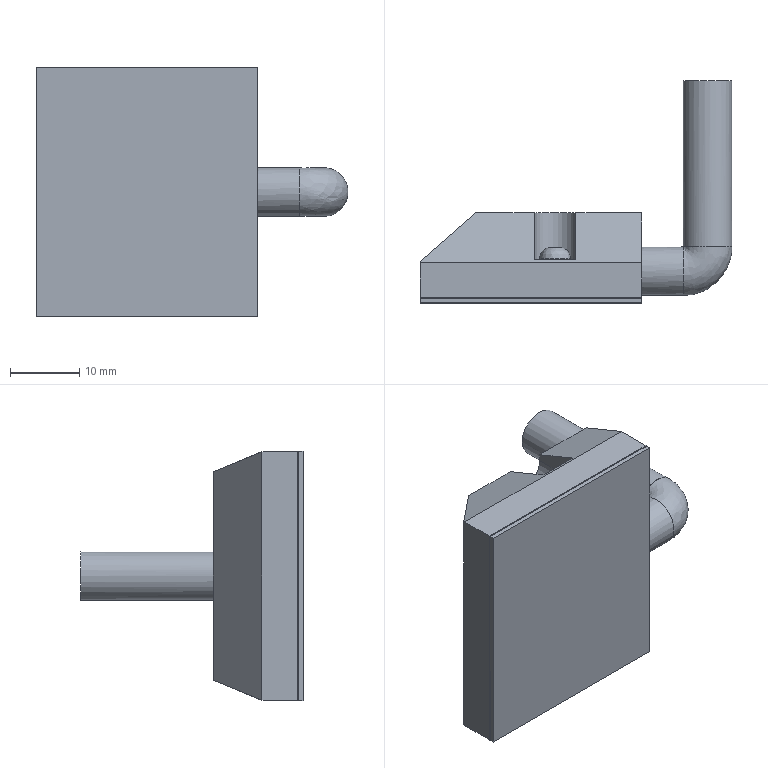Part | NX | 1 solid | 43 faces | box 45.035 x 32.1 x 36 mm | volume 14420 mm3 | plane 33 | cylinder 7 | spline 3 | commonest cylinder face diameters 4.5 x2 6 x2 7 x2 7.2 x1
STEP:
#1=CARTESIAN_POINT('',(-61.5,30.,-18.));
#2=VERTEX_POINT('',#1);
#3=CARTESIAN_POINT('',(-61.5,30.,18.));
#4=VERTEX_POINT('',#3);
#5=CARTESIAN_POINT('',(-61.5,30.,18.));
#6=DIRECTION('',(0.,0.,-1.));
#7=VECTOR('',#6,1000.);
#8=LINE('',#5,#7);
#9=EDGE_CURVE('',#2,#4,#8,.F.);
#10=ORIENTED_EDGE('',*,*,#9,.T.);
#11=CARTESIAN_POINT('',(-93.5,30.,18.));
#12=VERTEX_POINT('',#11);
#13=CARTESIAN_POINT('',(-61.5,30.,18.));
#14=DIRECTION('',(1.,0.,0.));
#15=VECTOR('',#14,1000.);
#16=LINE('',#13,#15);
#17=EDGE_CURVE('',#4,#12,#16,.F.);
#18=ORIENTED_EDGE('',*,*,#17,.T.);
#19=CARTESIAN_POINT('',(-93.5,30.,-18.));
#20=VERTEX_POINT('',#19);
#21=CARTESIAN_POINT('',(-93.5,30.,18.));
#22=DIRECTION('',(0.,0.,-1.));
#23=VECTOR('',#22,1000.);
#24=LINE('',#21,#23);
#25=EDGE_CURVE('',#12,#20,#24,.T.);
#26=ORIENTED_EDGE('',*,*,#25,.T.);
#27=CARTESIAN_POINT('',(-61.5,30.,-18.));
#28=DIRECTION('',(1.,0.,0.));
#29=VECTOR('',#28,1000.);
#30=LINE('',#27,#29);
#31=EDGE_CURVE('',#20,#2,#30,.T.);
#32=ORIENTED_EDGE('',*,*,#31,.T.);
#33=EDGE_LOOP('',(#10,#18,#26,#32));
#34=FACE_BOUND('',#33,.T.);
#35=CARTESIAN_POINT('',(-61.5,30.,18.));
#36=DIRECTION('',(0.,-1.,0.));
#37=DIRECTION('',(0.,0.,-1.));
#38=AXIS2_PLACEMENT_3D('',#35,#36,#37);
#39=PLANE('',#38);
#40=ADVANCED_FACE('',(#34),#39,.T.);
#41=CARTESIAN_POINT('',(-61.5,30.7,18.));
#42=VERTEX_POINT('',#41);
#43=CARTESIAN_POINT('',(-61.5,30.7,18.));
#44=DIRECTION('',(0.,1.,0.));
#45=VECTOR('',#44,1000.);
#46=LINE('',#43,#45);
#47=EDGE_CURVE('',#4,#42,#46,.T.);
#48=ORIENTED_EDGE('',*,*,#47,.T.);
#49=CARTESIAN_POINT('',(-93.5,30.7,18.));
#50=VERTEX_POINT('',#49);
#51=CARTESIAN_POINT('',(-61.5,30.7,18.));
#52=DIRECTION('',(1.,0.,0.));
#53=VECTOR('',#52,1000.);
#54=LINE('',#51,#53);
#55=EDGE_CURVE('',#42,#50,#54,.F.);
#56=ORIENTED_EDGE('',*,*,#55,.T.);
#57=CARTESIAN_POINT('',(-93.5,30.7,18.));
#58=DIRECTION('',(0.,1.,0.));
#59=VECTOR('',#58,1000.);
#60=LINE('',#57,#59);
#61=EDGE_CURVE('',#50,#12,#60,.F.);
#62=ORIENTED_EDGE('',*,*,#61,.T.);
#63=ORIENTED_EDGE('',*,*,#17,.F.);
#64=EDGE_LOOP('',(#48,#56,#62,#63));
#65=FACE_BOUND('',#64,.T.);
#66=CARTESIAN_POINT('',(-61.5,30.7,18.));
#67=DIRECTION('',(0.,0.,1.));
#68=DIRECTION('',(1.,0.,0.));
#69=AXIS2_PLACEMENT_3D('',#66,#67,#68);
#70=PLANE('',#69);
#71=ADVANCED_FACE('',(#65),#70,.T.);
#72=ORIENTED_EDGE('',*,*,#47,.F.);
#73=ORIENTED_EDGE('',*,*,#9,.F.);
#74=CARTESIAN_POINT('',(-61.5,30.7,-18.));
#75=VERTEX_POINT('',#74);
#76=CARTESIAN_POINT('',(-61.5,30.,-18.));
#77=DIRECTION('',(0.,1.,0.));
#78=VECTOR('',#77,1000.);
#79=LINE('',#76,#78);
#80=EDGE_CURVE('',#75,#2,#79,.F.);
#81=ORIENTED_EDGE('',*,*,#80,.F.);
#82=CARTESIAN_POINT('',(-61.5,30.7,0.));
#83=DIRECTION('',(0.,0.,1.));
#84=VECTOR('',#83,1000.);
#85=LINE('',#82,#84);
#86=EDGE_CURVE('',#42,#75,#85,.F.);
#87=ORIENTED_EDGE('',*,*,#86,.F.);
#88=EDGE_LOOP('',(#72,#73,#81,#87));
#89=FACE_BOUND('',#88,.T.);
#90=CARTESIAN_POINT('',(-61.5,30.,0.));
#91=DIRECTION('',(-1.,0.,0.));
#92=DIRECTION('',(0.,0.,1.));
#93=AXIS2_PLACEMENT_3D('',#90,#91,#92);
#94=PLANE('',#93);
#95=ADVANCED_FACE('',(#89),#94,.F.);
#96=ORIENTED_EDGE('',*,*,#80,.T.);
#97=ORIENTED_EDGE('',*,*,#31,.F.);
#98=CARTESIAN_POINT('',(-93.5,30.7,-18.));
#99=VERTEX_POINT('',#98);
#100=CARTESIAN_POINT('',(-93.5,30.,-18.));
#101=DIRECTION('',(0.,1.,0.));
#102=VECTOR('',#101,1000.);
#103=LINE('',#100,#102);
#104=EDGE_CURVE('',#20,#99,#103,.T.);
#105=ORIENTED_EDGE('',*,*,#104,.T.);
#106=CARTESIAN_POINT('',(-61.5,30.7,-18.));
#107=DIRECTION('',(-1.,0.,0.));
#108=VECTOR('',#107,1000.);
#109=LINE('',#106,#108);
#110=EDGE_CURVE('',#99,#75,#109,.F.);
#111=ORIENTED_EDGE('',*,*,#110,.T.);
#112=EDGE_LOOP('',(#96,#97,#105,#111));
#113=FACE_BOUND('',#112,.T.);
#114=CARTESIAN_POINT('',(-61.5,30.,-18.));
#115=DIRECTION('',(0.,0.,-1.));
#116=DIRECTION('',(-1.,0.,0.));
#117=AXIS2_PLACEMENT_3D('',#114,#115,#116);
#118=PLANE('',#117);
#119=ADVANCED_FACE('',(#113),#118,.T.);
#120=ORIENTED_EDGE('',*,*,#25,.F.);
#121=ORIENTED_EDGE('',*,*,#61,.F.);
#122=CARTESIAN_POINT('',(-93.5,30.7,0.));
#123=DIRECTION('',(0.,0.,1.));
#124=VECTOR('',#123,1000.);
#125=LINE('',#122,#124);
#126=EDGE_CURVE('',#50,#99,#125,.F.);
#127=ORIENTED_EDGE('',*,*,#126,.T.);
#128=ORIENTED_EDGE('',*,*,#104,.F.);
#129=EDGE_LOOP('',(#120,#121,#127,#128));
#130=FACE_BOUND('',#129,.T.);
#131=CARTESIAN_POINT('',(-93.5,30.,0.));
#132=DIRECTION('',(-1.,0.,0.));
#133=DIRECTION('',(0.,0.,1.));
#134=AXIS2_PLACEMENT_3D('',#131,#132,#133);
#135=PLANE('',#134);
#136=ADVANCED_FACE('',(#130),#135,.T.);
#137=ORIENTED_EDGE('',*,*,#86,.T.);
#138=ORIENTED_EDGE('',*,*,#110,.F.);
#139=ORIENTED_EDGE('',*,*,#126,.F.);
#140=ORIENTED_EDGE('',*,*,#55,.F.);
#141=EDGE_LOOP('',(#137,#138,#139,#140));
#142=FACE_BOUND('',#141,.T.);
#143=CARTESIAN_POINT('',(-61.6,30.7,17.9));
#144=VERTEX_POINT('',#143);
#145=CARTESIAN_POINT('',(-93.4,30.7,17.9));
#146=VERTEX_POINT('',#145);
#147=CARTESIAN_POINT('',(-61.5,30.7,17.9));
#148=DIRECTION('',(1.,0.,0.));
#149=VECTOR('',#148,1000.);
#150=LINE('',#147,#149);
#151=EDGE_CURVE('',#144,#146,#150,.F.);
#152=ORIENTED_EDGE('',*,*,#151,.T.);
#153=CARTESIAN_POINT('',(-93.4,30.7,-17.9));
#154=VERTEX_POINT('',#153);
#155=CARTESIAN_POINT('',(-93.4,30.7,-18.));
#156=DIRECTION('',(0.,0.,1.));
#157=VECTOR('',#156,1000.);
#158=LINE('',#155,#157);
#159=EDGE_CURVE('',#146,#154,#158,.F.);
#160=ORIENTED_EDGE('',*,*,#159,.T.);
#161=CARTESIAN_POINT('',(-61.6,30.7,-17.9));
#162=VERTEX_POINT('',#161);
#163=CARTESIAN_POINT('',(-61.5,30.7,-17.9));
#164=DIRECTION('',(1.,0.,0.));
#165=VECTOR('',#164,1000.);
#166=LINE('',#163,#165);
#167=EDGE_CURVE('',#154,#162,#166,.T.);
#168=ORIENTED_EDGE('',*,*,#167,.T.);
#169=CARTESIAN_POINT('',(-61.6,30.7,-18.));
#170=DIRECTION('',(0.,0.,1.));
#171=VECTOR('',#170,1000.);
#172=LINE('',#169,#171);
#173=EDGE_CURVE('',#162,#144,#172,.T.);
#174=ORIENTED_EDGE('',*,*,#173,.T.);
#175=EDGE_LOOP('',(#152,#160,#168,#174));
#176=FACE_BOUND('',#175,.T.);
#177=CARTESIAN_POINT('',(-61.5,30.7,-18.));
#178=DIRECTION('',(0.,1.,0.));
#179=DIRECTION('',(0.,0.,1.));
#180=AXIS2_PLACEMENT_3D('',#177,#178,#179);
#181=PLANE('',#180);
#182=ADVANCED_FACE('',(#142,#176),#181,.T.);
#183=CARTESIAN_POINT('',(-93.4,30.8,17.9));
#184=VERTEX_POINT('',#183);
#185=CARTESIAN_POINT('',(-93.4,30.,17.9));
#186=DIRECTION('',(0.,1.,0.));
#187=VECTOR('',#186,1000.);
#188=LINE('',#185,#187);
#189=EDGE_CURVE('',#146,#184,#188,.T.);
#190=ORIENTED_EDGE('',*,*,#189,.T.);
#191=CARTESIAN_POINT('',(-93.4,30.8,-17.9));
#192=VERTEX_POINT('',#191);
#193=CARTESIAN_POINT('',(-93.4,30.8,0.));
#194=DIRECTION('',(0.,0.,1.));
#195=VECTOR('',#194,1000.);
#196=LINE('',#193,#195);
#197=EDGE_CURVE('',#184,#192,#196,.F.);
#198=ORIENTED_EDGE('',*,*,#197,.T.);
#199=CARTESIAN_POINT('',(-93.4,30.,-17.9));
#200=DIRECTION('',(0.,1.,0.));
#201=VECTOR('',#200,1000.);
#202=LINE('',#199,#201);
#203=EDGE_CURVE('',#192,#154,#202,.F.);
#204=ORIENTED_EDGE('',*,*,#203,.T.);
#205=ORIENTED_EDGE('',*,*,#159,.F.);
#206=EDGE_LOOP('',(#190,#198,#204,#205));
#207=FACE_BOUND('',#206,.T.);
#208=CARTESIAN_POINT('',(-93.4,30.,0.));
#209=DIRECTION('',(-1.,0.,0.));
#210=DIRECTION('',(0.,0.,1.));
#211=AXIS2_PLACEMENT_3D('',#208,#209,#210);
#212=PLANE('',#211);
#213=ADVANCED_FACE('',(#207),#212,.T.);
#214=CARTESIAN_POINT('',(-61.6,30.8,17.9));
#215=VERTEX_POINT('',#214);
#216=CARTESIAN_POINT('',(-61.6,30.8,17.9));
#217=DIRECTION('',(0.,1.,0.));
#218=VECTOR('',#217,1000.);
#219=LINE('',#216,#218);
#220=EDGE_CURVE('',#144,#215,#219,.T.);
#221=ORIENTED_EDGE('',*,*,#220,.T.);
#222=CARTESIAN_POINT('',(-61.5,30.8,17.9));
#223=DIRECTION('',(1.,0.,0.));
#224=VECTOR('',#223,1000.);
#225=LINE('',#222,#224);
#226=EDGE_CURVE('',#215,#184,#225,.F.);
#227=ORIENTED_EDGE('',*,*,#226,.T.);
#228=ORIENTED_EDGE('',*,*,#189,.F.);
#229=ORIENTED_EDGE('',*,*,#151,.F.);
#230=EDGE_LOOP('',(#221,#227,#228,#229));
#231=FACE_BOUND('',#230,.T.);
#232=CARTESIAN_POINT('',(-61.5,30.8,17.9));
#233=DIRECTION('',(0.,0.,1.));
#234=DIRECTION('',(1.,0.,0.));
#235=AXIS2_PLACEMENT_3D('',#232,#233,#234);
#236=PLANE('',#235);
#237=ADVANCED_FACE('',(#231),#236,.T.);
#238=CARTESIAN_POINT('',(-61.6,30.8,-3.6));
#239=VERTEX_POINT('',#238);
#240=CARTESIAN_POINT('',(-61.6,30.8,-17.9));
#241=VERTEX_POINT('',#240);
#242=CARTESIAN_POINT('',(-61.6,30.8,0.));
#243=DIRECTION('',(0.,0.,1.));
#244=VECTOR('',#243,1000.);
#245=LINE('',#242,#244);
#246=EDGE_CURVE('',#239,#241,#245,.F.);
#247=ORIENTED_EDGE('',*,*,#246,.F.);
#248=CARTESIAN_POINT('',(-61.6,34.6,-3.6));
#249=VERTEX_POINT('',#248);
#250=CARTESIAN_POINT('',(-61.6,30.,-3.6));
#251=DIRECTION('',(0.,1.,0.));
#252=VECTOR('',#251,1000.);
#253=LINE('',#250,#252);
#254=EDGE_CURVE('',#249,#239,#253,.F.);
#255=ORIENTED_EDGE('',*,*,#254,.F.);
#256=CARTESIAN_POINT('',(-61.6,34.6,3.6));
#257=VERTEX_POINT('',#256);
#258=CARTESIAN_POINT('',(-61.6,34.6,0.));
#259=DIRECTION('',(1.,0.,0.));
#260=DIRECTION('',(0.,0.,-1.));
#261=AXIS2_PLACEMENT_3D('',#258,#259,#260);
#262=CIRCLE('',#261,3.6);
#263=EDGE_CURVE('',#257,#249,#262,.F.);
#264=ORIENTED_EDGE('',*,*,#263,.F.);
#265=CARTESIAN_POINT('',(-61.6,30.8,3.6));
#266=VERTEX_POINT('',#265);
#267=CARTESIAN_POINT('',(-61.6,30.,3.6));
#268=DIRECTION('',(0.,1.,0.));
#269=VECTOR('',#268,1000.);
#270=LINE('',#267,#269);
#271=EDGE_CURVE('',#266,#257,#270,.T.);
#272=ORIENTED_EDGE('',*,*,#271,.F.);
#273=CARTESIAN_POINT('',(-61.6,30.8,0.));
#274=DIRECTION('',(0.,0.,1.));
#275=VECTOR('',#274,1000.);
#276=LINE('',#273,#275);
#277=EDGE_CURVE('',#215,#266,#276,.F.);
#278=ORIENTED_EDGE('',*,*,#277,.F.);
#279=ORIENTED_EDGE('',*,*,#220,.F.);
#280=ORIENTED_EDGE('',*,*,#173,.F.);
#281=CARTESIAN_POINT('',(-61.6,30.,-17.9));
#282=DIRECTION('',(0.,1.,0.));
#283=VECTOR('',#282,1000.);
#284=LINE('',#281,#283);
#285=EDGE_CURVE('',#241,#162,#284,.F.);
#286=ORIENTED_EDGE('',*,*,#285,.F.);
#287=EDGE_LOOP('',(#247,#255,#264,#272,#278,#279,#280,#286));
#288=FACE_BOUND('',#287,.T.);
#289=CARTESIAN_POINT('',(-61.6,34.6,-3.5));
#290=VERTEX_POINT('',#289);
#291=CARTESIAN_POINT('',(-61.6,34.6,0.));
#292=DIRECTION('',(1.,0.,0.));
#293=DIRECTION('',(0.,0.,-1.));
#294=AXIS2_PLACEMENT_3D('',#291,#292,#293);
#295=CIRCLE('',#294,3.5);
#296=EDGE_CURVE('',#290,#290,#295,.T.);
#297=ORIENTED_EDGE('',*,*,#296,.F.);
#298=EDGE_LOOP('',(#297));
#299=FACE_BOUND('',#298,.T.);
#300=CARTESIAN_POINT('',(-61.6,30.,0.));
#301=DIRECTION('',(-1.,0.,0.));
#302=DIRECTION('',(0.,0.,1.));
#303=AXIS2_PLACEMENT_3D('',#300,#301,#302);
#304=PLANE('',#303);
#305=ADVANCED_FACE('',(#288,#299),#304,.F.);
#306=ORIENTED_EDGE('',*,*,#285,.T.);
#307=ORIENTED_EDGE('',*,*,#167,.F.);
#308=ORIENTED_EDGE('',*,*,#203,.F.);
#309=CARTESIAN_POINT('',(-61.5,30.8,-17.9));
#310=DIRECTION('',(1.,0.,0.));
#311=VECTOR('',#310,1000.);
#312=LINE('',#309,#311);
#313=EDGE_CURVE('',#192,#241,#312,.T.);
#314=ORIENTED_EDGE('',*,*,#313,.T.);
#315=EDGE_LOOP('',(#306,#307,#308,#314));
#316=FACE_BOUND('',#315,.T.);
#317=CARTESIAN_POINT('',(-61.5,30.7,-17.9));
#318=DIRECTION('',(0.,0.,-1.));
#319=DIRECTION('',(0.,1.,0.));
#320=AXIS2_PLACEMENT_3D('',#317,#318,#319);
#321=PLANE('',#320);
#322=ADVANCED_FACE('',(#316),#321,.T.);
#323=CARTESIAN_POINT('',(-93.5,30.8,-18.));
#324=VERTEX_POINT('',#323);
#325=CARTESIAN_POINT('',(-61.5,30.8,-18.));
#326=VERTEX_POINT('',#325);
#327=CARTESIAN_POINT('',(-61.5,30.8,-18.));
#328=DIRECTION('',(1.,0.,0.));
#329=VECTOR('',#328,1000.);
#330=LINE('',#327,#329);
#331=EDGE_CURVE('',#324,#326,#330,.T.);
#332=ORIENTED_EDGE('',*,*,#331,.T.);
#333=CARTESIAN_POINT('',(-61.5,30.8,-3.6));
#334=VERTEX_POINT('',#333);
#335=CARTESIAN_POINT('',(-61.5,30.8,-17.9));
#336=DIRECTION('',(0.,0.,-1.));
#337=VECTOR('',#336,1000.);
#338=LINE('',#335,#337);
#339=EDGE_CURVE('',#326,#334,#338,.F.);
#340=ORIENTED_EDGE('',*,*,#339,.T.);
#341=CARTESIAN_POINT('',(-61.5,30.8,-3.6));
#342=DIRECTION('',(1.,0.,0.));
#343=VECTOR('',#342,1000.);
#344=LINE('',#341,#343);
#345=EDGE_CURVE('',#334,#239,#344,.F.);
#346=ORIENTED_EDGE('',*,*,#345,.T.);
#347=ORIENTED_EDGE('',*,*,#246,.T.);
#348=ORIENTED_EDGE('',*,*,#313,.F.);
#349=ORIENTED_EDGE('',*,*,#197,.F.);
#350=ORIENTED_EDGE('',*,*,#226,.F.);
#351=ORIENTED_EDGE('',*,*,#277,.T.);
#352=CARTESIAN_POINT('',(-61.5,30.8,3.6));
#353=VERTEX_POINT('',#352);
#354=CARTESIAN_POINT('',(-61.5,30.8,3.6));
#355=DIRECTION('',(1.,0.,0.));
#356=VECTOR('',#355,1000.);
#357=LINE('',#354,#356);
#358=EDGE_CURVE('',#266,#353,#357,.T.);
#359=ORIENTED_EDGE('',*,*,#358,.T.);
#360=CARTESIAN_POINT('',(-61.5,30.8,18.));
#361=VERTEX_POINT('',#360);
#362=CARTESIAN_POINT('',(-61.5,30.8,-17.9));
#363=DIRECTION('',(0.,0.,-1.));
#364=VECTOR('',#363,1000.);
#365=LINE('',#362,#364);
#366=EDGE_CURVE('',#353,#361,#365,.F.);
#367=ORIENTED_EDGE('',*,*,#366,.T.);
#368=CARTESIAN_POINT('',(-93.5,30.8,18.));
#369=VERTEX_POINT('',#368);
#370=CARTESIAN_POINT('',(-61.5,30.8,18.));
#371=DIRECTION('',(1.,0.,0.));
#372=VECTOR('',#371,1000.);
#373=LINE('',#370,#372);
#374=EDGE_CURVE('',#361,#369,#373,.F.);
#375=ORIENTED_EDGE('',*,*,#374,.T.);
#376=CARTESIAN_POINT('',(-93.5,30.8,-17.9));
#377=DIRECTION('',(0.,0.,-1.));
#378=VECTOR('',#377,1000.);
#379=LINE('',#376,#378);
#380=EDGE_CURVE('',#369,#324,#379,.T.);
#381=ORIENTED_EDGE('',*,*,#380,.T.);
#382=EDGE_LOOP('',(#332,#340,#346,#347,#348,#349,#350,#351,#359,#367,#375,#381));
#383=FACE_BOUND('',#382,.T.);
#384=CARTESIAN_POINT('',(-61.5,30.8,-17.9));
#385=DIRECTION('',(0.,-1.,0.));
#386=DIRECTION('',(0.,0.,-1.));
#387=AXIS2_PLACEMENT_3D('',#384,#385,#386);
#388=PLANE('',#387);
#389=ADVANCED_FACE('',(#383),#388,.T.);
#390=ORIENTED_EDGE('',*,*,#345,.F.);
#391=CARTESIAN_POINT('',(-61.5,34.6,-3.6));
#392=VERTEX_POINT('',#391);
#393=CARTESIAN_POINT('',(-61.5,30.8,-3.6));
#394=DIRECTION('',(0.,1.,0.));
#395=VECTOR('',#394,1000.);
#396=LINE('',#393,#395);
#397=EDGE_CURVE('',#392,#334,#396,.F.);
#398=ORIENTED_EDGE('',*,*,#397,.F.);
#399=CARTESIAN_POINT('',(-61.5,34.6,-3.6));
#400=DIRECTION('',(-1.,0.,0.));
#401=VECTOR('',#400,1000.);
#402=LINE('',#399,#401);
#403=EDGE_CURVE('',#249,#392,#402,.F.);
#404=ORIENTED_EDGE('',*,*,#403,.F.);
#405=ORIENTED_EDGE('',*,*,#254,.T.);
#406=EDGE_LOOP('',(#390,#398,#404,#405));
#407=FACE_BOUND('',#406,.T.);
#408=CARTESIAN_POINT('',(-61.5,30.8,-3.6));
#409=DIRECTION('',(0.,0.,-1.));
#410=DIRECTION('',(-1.,0.,0.));
#411=AXIS2_PLACEMENT_3D('',#408,#409,#410);
#412=PLANE('',#411);
#413=ADVANCED_FACE('',(#407),#412,.F.);
#414=ORIENTED_EDGE('',*,*,#403,.T.);
#415=CARTESIAN_POINT('',(-61.5,34.6,3.6));
#416=VERTEX_POINT('',#415);
#417=CARTESIAN_POINT('',(-61.5,34.6,0.));
#418=DIRECTION('',(1.,0.,0.));
#419=DIRECTION('',(0.,0.,-1.));
#420=AXIS2_PLACEMENT_3D('',#417,#418,#419);
#421=CIRCLE('',#420,3.6);
#422=EDGE_CURVE('',#416,#392,#421,.F.);
#423=ORIENTED_EDGE('',*,*,#422,.F.);
#424=CARTESIAN_POINT('',(-61.5,34.6,3.6));
#425=DIRECTION('',(1.,0.,0.));
#426=VECTOR('',#425,1000.);
#427=LINE('',#424,#426);
#428=EDGE_CURVE('',#257,#416,#427,.T.);
#429=ORIENTED_EDGE('',*,*,#428,.F.);
#430=ORIENTED_EDGE('',*,*,#263,.T.);
#431=EDGE_LOOP('',(#414,#423,#429,#430));
#432=FACE_BOUND('',#431,.T.);
#433=CARTESIAN_POINT('',(-61.5,34.6,0.));
#434=DIRECTION('',(1.,0.,0.));
#435=DIRECTION('',(0.,0.,-1.));
#436=AXIS2_PLACEMENT_3D('',#433,#434,#435);
#437=CYLINDRICAL_SURFACE('',#436,3.6);
#438=ADVANCED_FACE('',(#432),#437,.F.);
#439=ORIENTED_EDGE('',*,*,#428,.T.);
#440=CARTESIAN_POINT('',(-61.5,34.6,3.6));
#441=DIRECTION('',(0.,1.,0.));
#442=VECTOR('',#441,1000.);
#443=LINE('',#440,#442);
#444=EDGE_CURVE('',#353,#416,#443,.T.);
#445=ORIENTED_EDGE('',*,*,#444,.F.);
#446=ORIENTED_EDGE('',*,*,#358,.F.);
#447=ORIENTED_EDGE('',*,*,#271,.T.);
#448=EDGE_LOOP('',(#439,#445,#446,#447));
#449=FACE_BOUND('',#448,.T.);
#450=CARTESIAN_POINT('',(-61.5,34.6,3.6));
#451=DIRECTION('',(0.,0.,1.));
#452=DIRECTION('',(1.,0.,0.));
#453=AXIS2_PLACEMENT_3D('',#450,#451,#452);
#454=PLANE('',#453);
#455=ADVANCED_FACE('',(#449),#454,.F.);
#456=CARTESIAN_POINT('',(-55.5,38.1,0.));
#457=VERTEX_POINT('',#456);
#458=CARTESIAN_POINT('',(-55.5,34.6,0.));
#459=DIRECTION('',(1.,0.,0.));
#460=DIRECTION('',(0.,0.,-1.));
#461=AXIS2_PLACEMENT_3D('',#458,#459,#460);
#462=CIRCLE('',#461,3.5);
#463=EDGE_CURVE('',#457,#457,#462,.F.);
#464=ORIENTED_EDGE('',*,*,#463,.T.);
#465=EDGE_LOOP('',(#464));
#466=FACE_BOUND('',#465,.T.);
#467=ORIENTED_EDGE('',*,*,#296,.T.);
#468=EDGE_LOOP('',(#467));
#469=FACE_BOUND('',#468,.T.);
#470=CARTESIAN_POINT('',(-55.5,34.6,0.));
#471=DIRECTION('',(1.,0.,0.));
#472=DIRECTION('',(0.,0.,-1.));
#473=AXIS2_PLACEMENT_3D('',#470,#471,#472);
#474=CYLINDRICAL_SURFACE('',#473,3.5);
#475=ADVANCED_FACE('',(#466,#469),#474,.T.);
#476=ORIENTED_EDGE('',*,*,#339,.F.);
#477=CARTESIAN_POINT('',(-61.5,35.8,-18.));
#478=VERTEX_POINT('',#477);
#479=CARTESIAN_POINT('',(-61.5,30.,-18.));
#480=DIRECTION('',(0.,1.,0.));
#481=VECTOR('',#480,1000.);
#482=LINE('',#479,#481);
#483=EDGE_CURVE('',#478,#326,#482,.F.);
#484=ORIENTED_EDGE('',*,*,#483,.F.);
#485=CARTESIAN_POINT('',(-61.5,43.,-15.041));
#486=VERTEX_POINT('',#485);
#487=CARTESIAN_POINT('',(-61.5,43.,-15.041));
#488=DIRECTION('',(0.,-0.9249,-0.3801));
#489=VECTOR('',#488,1000.);
#490=LINE('',#487,#489);
#491=EDGE_CURVE('',#486,#478,#490,.T.);
#492=ORIENTED_EDGE('',*,*,#491,.F.);
#493=CARTESIAN_POINT('',(-61.5,43.,15.041));
#494=VERTEX_POINT('',#493);
#495=CARTESIAN_POINT('',(-61.5,43.,0.));
#496=DIRECTION('',(0.,0.,1.));
#497=VECTOR('',#496,1000.);
#498=LINE('',#495,#497);
#499=EDGE_CURVE('',#494,#486,#498,.F.);
#500=ORIENTED_EDGE('',*,*,#499,.F.);
#501=CARTESIAN_POINT('',(-61.5,35.8,18.));
#502=VERTEX_POINT('',#501);
#503=CARTESIAN_POINT('',(-61.5,35.8,18.));
#504=DIRECTION('',(0.,0.9249,-0.3801));
#505=VECTOR('',#504,1000.);
#506=LINE('',#503,#505);
#507=EDGE_CURVE('',#502,#494,#506,.T.);
#508=ORIENTED_EDGE('',*,*,#507,.F.);
#509=CARTESIAN_POINT('',(-61.5,30.,18.));
#510=DIRECTION('',(0.,1.,0.));
#511=VECTOR('',#510,1000.);
#512=LINE('',#509,#511);
#513=EDGE_CURVE('',#361,#502,#512,.T.);
#514=ORIENTED_EDGE('',*,*,#513,.F.);
#515=ORIENTED_EDGE('',*,*,#366,.F.);
#516=ORIENTED_EDGE('',*,*,#444,.T.);
#517=ORIENTED_EDGE('',*,*,#422,.T.);
#518=ORIENTED_EDGE('',*,*,#397,.T.);
#519=EDGE_LOOP('',(#476,#484,#492,#500,#508,#514,#515,#516,#517,#518));
#520=FACE_BOUND('',#519,.T.);
#521=CARTESIAN_POINT('',(-61.5,30.,0.));
#522=DIRECTION('',(-1.,0.,0.));
#523=DIRECTION('',(0.,0.,1.));
#524=AXIS2_PLACEMENT_3D('',#521,#522,#523);
#525=PLANE('',#524);
#526=ADVANCED_FACE('',(#520),#525,.F.);
#527=ORIENTED_EDGE('',*,*,#483,.T.);
#528=ORIENTED_EDGE('',*,*,#331,.F.);
#529=CARTESIAN_POINT('',(-93.5,35.8,-18.));
#530=VERTEX_POINT('',#529);
#531=CARTESIAN_POINT('',(-93.5,30.8,-18.));
#532=DIRECTION('',(0.,1.,0.));
#533=VECTOR('',#532,1000.);
#534=LINE('',#531,#533);
#535=EDGE_CURVE('',#324,#530,#534,.T.);
#536=ORIENTED_EDGE('',*,*,#535,.T.);
#537=CARTESIAN_POINT('',(-61.5,35.8,-18.));
#538=DIRECTION('',(-1.,0.,0.));
#539=VECTOR('',#538,1000.);
#540=LINE('',#537,#539);
#541=EDGE_CURVE('',#530,#478,#540,.F.);
#542=ORIENTED_EDGE('',*,*,#541,.T.);
#543=EDGE_LOOP('',(#527,#528,#536,#542));
#544=FACE_BOUND('',#543,.T.);
#545=CARTESIAN_POINT('',(-61.5,30.8,-18.));
#546=DIRECTION('',(0.,0.,-1.));
#547=DIRECTION('',(-1.,0.,0.));
#548=AXIS2_PLACEMENT_3D('',#545,#546,#547);
#549=PLANE('',#548);
#550=ADVANCED_FACE('',(#544),#549,.T.);
#551=CARTESIAN_POINT('',(-93.5,35.8,18.));
#552=VERTEX_POINT('',#551);
#553=CARTESIAN_POINT('',(-93.5,30.,18.));
#554=DIRECTION('',(0.,1.,0.));
#555=VECTOR('',#554,1000.);
#556=LINE('',#553,#555);
#557=EDGE_CURVE('',#369,#552,#556,.T.);
#558=ORIENTED_EDGE('',*,*,#557,.T.);
#559=CARTESIAN_POINT('',(-93.5,36.,17.918));
#560=VERTEX_POINT('',#559);
#561=CARTESIAN_POINT('',(-93.5,35.8,18.));
#562=DIRECTION('',(0.,0.9249,-0.3801));
#563=VECTOR('',#562,1000.);
#564=LINE('',#561,#563);
#565=EDGE_CURVE('',#552,#560,#564,.T.);
#566=ORIENTED_EDGE('',*,*,#565,.T.);
#567=CARTESIAN_POINT('',(-93.5,36.,-17.918));
#568=VERTEX_POINT('',#567);
#569=CARTESIAN_POINT('',(-93.5,36.,0.));
#570=DIRECTION('',(0.,0.,1.));
#571=VECTOR('',#570,1000.);
#572=LINE('',#569,#571);
#573=EDGE_CURVE('',#560,#568,#572,.F.);
#574=ORIENTED_EDGE('',*,*,#573,.T.);
#575=CARTESIAN_POINT('',(-93.5,36.,-17.918));
#576=DIRECTION('',(0.,-0.9249,-0.3801));
#577=VECTOR('',#576,1000.);
#578=LINE('',#575,#577);
#579=EDGE_CURVE('',#568,#530,#578,.T.);
#580=ORIENTED_EDGE('',*,*,#579,.T.);
#581=ORIENTED_EDGE('',*,*,#535,.F.);
#582=ORIENTED_EDGE('',*,*,#380,.F.);
#583=EDGE_LOOP('',(#558,#566,#574,#580,#581,#582));
#584=FACE_BOUND('',#583,.T.);
#585=CARTESIAN_POINT('',(-93.5,30.,0.));
#586=DIRECTION('',(-1.,0.,0.));
#587=DIRECTION('',(0.,0.,1.));
#588=AXIS2_PLACEMENT_3D('',#585,#586,#587);
#589=PLANE('',#588);
#590=ADVANCED_FACE('',(#584),#589,.T.);
#591=ORIENTED_EDGE('',*,*,#513,.T.);
#592=CARTESIAN_POINT('',(-61.5,35.8,18.));
#593=DIRECTION('',(1.,0.,0.));
#594=VECTOR('',#593,1000.);
#595=LINE('',#592,#594);
#596=EDGE_CURVE('',#502,#552,#595,.F.);
#597=ORIENTED_EDGE('',*,*,#596,.T.);
#598=ORIENTED_EDGE('',*,*,#557,.F.);
#599=ORIENTED_EDGE('',*,*,#374,.F.);
#600=EDGE_LOOP('',(#591,#597,#598,#599));
#601=FACE_BOUND('',#600,.T.);
#602=CARTESIAN_POINT('',(-61.5,35.8,18.));
#603=DIRECTION('',(0.,0.,1.));
#604=DIRECTION('',(1.,0.,0.));
#605=AXIS2_PLACEMENT_3D('',#602,#603,#604);
#606=PLANE('',#605);
#607=ADVANCED_FACE('',(#601),#606,.T.);
#608=CARTESIAN_POINT('',(-51.983,38.135,-3.5));
#609=VERTEX_POINT('',#608);
#610=CARTESIAN_POINT('',(-51.991,38.1,-3.5));
#611=VERTEX_POINT('',#610);
#612=CARTESIAN_POINT('',(-51.982,38.135,-3.5));
#613=CARTESIAN_POINT('',(-51.983,38.123,-3.5));
#614=CARTESIAN_POINT('',(-51.983,38.112,-3.5));
#615=CARTESIAN_POINT('',(-51.983,38.1,-3.5));
#616=B_SPLINE_CURVE_WITH_KNOTS('',3,(#612,#613,#614,#615),.UNSPECIFIED.,.F.,.F.,(4,4),(0.,1.),.UNSPECIFIED.);
#617=EDGE_CURVE('',#609,#611,#616,.T.);
#618=ORIENTED_EDGE('',*,*,#617,.F.);
#619=CARTESIAN_POINT('',(-51.983,38.135,3.5));
#620=VERTEX_POINT('',#619);
#621=CARTESIAN_POINT('',(-51.983,38.135,-3.5));
#622=CARTESIAN_POINT('',(-51.055,38.135,-3.505));
#623=CARTESIAN_POINT('',(-49.234,38.135,-2.753));
#624=CARTESIAN_POINT('',(-48.081,38.135,0.0008832));
#625=CARTESIAN_POINT('',(-49.231,38.135,2.749));
#626=CARTESIAN_POINT('',(-51.055,38.135,3.505));
#627=CARTESIAN_POINT('',(-51.983,38.135,3.5));
#628=B_SPLINE_CURVE_WITH_KNOTS('',3,(#621,#622,#623,#624,#625,#626,#627),.UNSPECIFIED.,.F.,.F.,(4,1,1,1,4),(0.,0.002743,0.005485,0.008228,0.01097),.UNSPECIFIED.);
#629=EDGE_CURVE('',#609,#620,#628,.T.);
#630=ORIENTED_EDGE('',*,*,#629,.T.);
#631=CARTESIAN_POINT('',(-51.991,38.1,3.5));
#632=VERTEX_POINT('',#631);
#633=CARTESIAN_POINT('',(-51.983,38.1,3.5));
#634=CARTESIAN_POINT('',(-51.983,38.112,3.5));
#635=CARTESIAN_POINT('',(-51.983,38.123,3.5));
#636=CARTESIAN_POINT('',(-51.983,38.135,3.5));
#637=B_SPLINE_CURVE_WITH_KNOTS('',3,(#633,#634,#635,#636),.UNSPECIFIED.,.F.,.F.,(4,4),(0.,1.),.UNSPECIFIED.);
#638=EDGE_CURVE('',#632,#620,#637,.T.);
#639=ORIENTED_EDGE('',*,*,#638,.F.);
#640=CARTESIAN_POINT('',(-51.991,38.1,3.5));
#641=CARTESIAN_POINT('',(-52.912,38.1,3.493));
#642=CARTESIAN_POINT('',(-54.252,38.1,2.916));
#643=CARTESIAN_POINT('',(-55.292,38.1,1.371));
#644=CARTESIAN_POINT('',(-55.455,38.1,0.4516));
#645=CARTESIAN_POINT('',(-55.5,38.1,0.));
#646=B_SPLINE_CURVE_WITH_KNOTS('',3,(#640,#641,#642,#643,#644,#645),.UNSPECIFIED.,.F.,.F.,(4,1,1,4),(0.,0.002723,0.004084,0.005446),.UNSPECIFIED.);
#647=EDGE_CURVE('',#632,#457,#646,.T.);
#648=ORIENTED_EDGE('',*,*,#647,.T.);
#649=ORIENTED_EDGE('',*,*,#463,.F.);
#650=CARTESIAN_POINT('',(-52.,38.1,-3.5));
#651=CARTESIAN_POINT('',(-52.461,38.1,-3.495));
#652=CARTESIAN_POINT('',(-53.359,38.1,-3.306));
#653=CARTESIAN_POINT('',(-54.516,38.1,-2.529));
#654=CARTESIAN_POINT('',(-55.155,38.1,-1.557));
#655=CARTESIAN_POINT('',(-55.39,38.1,-0.8039));
#656=CARTESIAN_POINT('',(-55.469,38.1,-0.3137));
#657=CARTESIAN_POINT('',(-55.485,38.1,-0.1451));
#658=CARTESIAN_POINT('',(-55.5,38.1,0.));
#659=B_SPLINE_CURVE_WITH_KNOTS('',3,(#650,#651,#652,#653,#654,#655,#656,#657,#658),.UNSPECIFIED.,.F.,.F.,(4,1,1,1,1,1,4),(0.003134,0.2524,0.5016,0.7508,0.8754,0.9377,1.),.UNSPECIFIED.);
#660=EDGE_CURVE('',#457,#611,#659,.F.);
#661=ORIENTED_EDGE('',*,*,#660,.T.);
#662=EDGE_LOOP('',(#618,#630,#639,#648,#649,#661));
#663=FACE_BOUND('',#662,.T.);
#664=CARTESIAN_POINT('',(-55.5,31.857,2.743));
#665=CARTESIAN_POINT('',(-51.795,31.857,2.743));
#666=CARTESIAN_POINT('',(-49.188,34.489,2.743));
#667=CARTESIAN_POINT('',(-49.223,38.194,2.743));
#668=CARTESIAN_POINT('',(-55.5,30.721,0.));
#669=CARTESIAN_POINT('',(-51.125,30.721,0.));
#670=CARTESIAN_POINT('',(-48.045,33.83,0.));
#671=CARTESIAN_POINT('',(-48.087,38.205,0.));
#672=CARTESIAN_POINT('',(-55.5,31.857,-2.743));
#673=CARTESIAN_POINT('',(-51.795,31.857,-2.743));
#674=CARTESIAN_POINT('',(-49.188,34.489,-2.743));
#675=CARTESIAN_POINT('',(-49.223,38.194,-2.743));
#676=CARTESIAN_POINT('',(-55.5,34.6,-3.879));
#677=CARTESIAN_POINT('',(-53.414,34.6,-3.879));
#678=CARTESIAN_POINT('',(-51.945,36.082,-3.879));
#679=CARTESIAN_POINT('',(-51.965,38.168,-3.879));
#680=CARTESIAN_POINT('',(-55.5,37.343,-2.743));
#681=CARTESIAN_POINT('',(-55.032,37.343,-2.743));
#682=CARTESIAN_POINT('',(-54.703,37.675,-2.743));
#683=CARTESIAN_POINT('',(-54.708,38.142,-2.743));
#684=CARTESIAN_POINT('',(-55.5,38.479,0.));
#685=CARTESIAN_POINT('',(-55.703,38.479,0.));
#686=CARTESIAN_POINT('',(-55.846,38.335,0.));
#687=CARTESIAN_POINT('',(-55.844,38.132,0.));
#688=CARTESIAN_POINT('',(-55.5,37.343,2.743));
#689=CARTESIAN_POINT('',(-55.032,37.343,2.743));
#690=CARTESIAN_POINT('',(-54.703,37.675,2.743));
#691=CARTESIAN_POINT('',(-54.708,38.142,2.743));
#692=CARTESIAN_POINT('',(-55.5,34.6,3.879));
#693=CARTESIAN_POINT('',(-53.414,34.6,3.879));
#694=CARTESIAN_POINT('',(-51.945,36.082,3.879));
#695=CARTESIAN_POINT('',(-51.965,38.168,3.879));
#696=CARTESIAN_POINT('',(-55.5,31.857,2.743));
#697=CARTESIAN_POINT('',(-51.795,31.857,2.743));
#698=CARTESIAN_POINT('',(-49.188,34.489,2.743));
#699=CARTESIAN_POINT('',(-49.223,38.194,2.743));
#700=CARTESIAN_POINT('',(-55.5,30.721,0.));
#701=CARTESIAN_POINT('',(-51.125,30.721,0.));
#702=CARTESIAN_POINT('',(-48.045,33.83,0.));
#703=CARTESIAN_POINT('',(-48.087,38.205,0.));
#704=CARTESIAN_POINT('',(-55.5,31.857,-2.743));
#705=CARTESIAN_POINT('',(-51.795,31.857,-2.743));
#706=CARTESIAN_POINT('',(-49.188,34.489,-2.743));
#707=CARTESIAN_POINT('',(-49.223,38.194,-2.743));
#708=(BOUNDED_SURFACE()B_SPLINE_SURFACE(3,3,((#664,#665,#666,#667),(#668,#669,#670,#671),(#672,#673,#674,#675),(#676,#677,#678,#679),(#680,#681,#682,#683),(#684,#685,#686,#687),(#688,#689,#690,#691),(#692,#693,#694,#695),(#696,#697,#698,#699),(#700,#701,#702,#703),(#704,#705,#706,#707)),.SURF_OF_REVOLUTION.,.T.,.F.,.F.)B_SPLINE_SURFACE_WITH_KNOTS((1,1,1,1,1,1,1,1,1,1,1,1,1,1,1),(4,4),(-2.356,-1.571,-0.7854,0.,0.7854,1.571,2.356,3.142,3.927,4.712,5.498,6.283,7.069,7.854,8.639),(0.,1.),.UNSPECIFIED.)GEOMETRIC_REPRESENTATION_ITEM()RATIONAL_B_SPLINE_SURFACE(((1.,0.8025,0.8025,1.),(1.,0.8025,0.8025,1.),(1.,0.8025,0.8025,1.),(1.,0.8025,0.8025,1.),(1.,0.8025,0.8025,1.),(1.,0.8025,0.8025,1.),(1.,0.8025,0.8025,1.),(1.,0.8025,0.8025,1.),(1.,0.8025,0.8025,1.),(1.,0.8025,0.8025,1.),(1.,0.8025,0.8025,1.)))REPRESENTATION_ITEM('')SURFACE());
#709=ADVANCED_FACE('',(#663),#708,.T.);
#710=CARTESIAN_POINT('',(-77.,43.,-15.041));
#711=VERTEX_POINT('',#710);
#712=CARTESIAN_POINT('',(-77.,36.3,-17.795));
#713=VERTEX_POINT('',#712);
#714=CARTESIAN_POINT('',(-77.,35.8,-18.));
#715=DIRECTION('',(0.,0.9249,0.3801));
#716=VECTOR('',#715,1000.);
#717=LINE('',#714,#716);
#718=EDGE_CURVE('',#711,#713,#717,.F.);
#719=ORIENTED_EDGE('',*,*,#718,.T.);
#720=CARTESIAN_POINT('',(-71.,36.3,-17.795));
#721=VERTEX_POINT('',#720);
#722=CARTESIAN_POINT('',(-61.5,36.3,-17.795));
#723=DIRECTION('',(1.,0.,0.));
#724=VECTOR('',#723,1000.);
#725=LINE('',#722,#724);
#726=EDGE_CURVE('',#713,#721,#725,.T.);
#727=ORIENTED_EDGE('',*,*,#726,.T.);
#728=CARTESIAN_POINT('',(-71.,43.,-15.041));
#729=VERTEX_POINT('',#728);
#730=CARTESIAN_POINT('',(-71.,35.8,-18.));
#731=DIRECTION('',(0.,0.9249,0.3801));
#732=VECTOR('',#731,1000.);
#733=LINE('',#730,#732);
#734=EDGE_CURVE('',#721,#729,#733,.T.);
#735=ORIENTED_EDGE('',*,*,#734,.T.);
#736=CARTESIAN_POINT('',(-61.5,43.,-15.041));
#737=DIRECTION('',(1.,0.,0.));
#738=VECTOR('',#737,1000.);
#739=LINE('',#736,#738);
#740=EDGE_CURVE('',#729,#486,#739,.T.);
#741=ORIENTED_EDGE('',*,*,#740,.T.);
#742=ORIENTED_EDGE('',*,*,#491,.T.);
#743=ORIENTED_EDGE('',*,*,#541,.F.);
#744=ORIENTED_EDGE('',*,*,#579,.F.);
#745=CARTESIAN_POINT('',(-85.5,43.,-15.041));
#746=VERTEX_POINT('',#745);
#747=CARTESIAN_POINT('',(-93.5,36.,-17.918));
#748=DIRECTION('',(0.7264,0.6356,0.2612));
#749=VECTOR('',#748,1000.);
#750=LINE('',#747,#749);
#751=EDGE_CURVE('',#568,#746,#750,.T.);
#752=ORIENTED_EDGE('',*,*,#751,.T.);
#753=CARTESIAN_POINT('',(-61.5,43.,-15.041));
#754=DIRECTION('',(1.,0.,0.));
#755=VECTOR('',#754,1000.);
#756=LINE('',#753,#755);
#757=EDGE_CURVE('',#746,#711,#756,.T.);
#758=ORIENTED_EDGE('',*,*,#757,.T.);
#759=EDGE_LOOP('',(#719,#727,#735,#741,#742,#743,#744,#752,#758));
#760=FACE_BOUND('',#759,.T.);
#761=CARTESIAN_POINT('',(-61.5,35.8,-18.));
#762=DIRECTION('',(0.,0.3801,-0.9249));
#763=DIRECTION('',(0.,0.9249,0.3801));
#764=AXIS2_PLACEMENT_3D('',#761,#762,#763);
#765=PLANE('',#764);
#766=ADVANCED_FACE('',(#760),#765,.T.);
#767=CARTESIAN_POINT('',(-85.5,43.,15.041));
#768=VERTEX_POINT('',#767);
#769=CARTESIAN_POINT('',(-85.5,43.,-15.041));
#770=DIRECTION('',(0.,0.,1.));
#771=VECTOR('',#770,1000.);
#772=LINE('',#769,#771);
#773=EDGE_CURVE('',#746,#768,#772,.T.);
#774=ORIENTED_EDGE('',*,*,#773,.T.);
#775=CARTESIAN_POINT('',(-77.,43.,15.041));
#776=VERTEX_POINT('',#775);
#777=CARTESIAN_POINT('',(-61.5,43.,15.041));
#778=DIRECTION('',(1.,0.,0.));
#779=VECTOR('',#778,1000.);
#780=LINE('',#777,#779);
#781=EDGE_CURVE('',#768,#776,#780,.T.);
#782=ORIENTED_EDGE('',*,*,#781,.T.);
#783=CARTESIAN_POINT('',(-77.,43.,14.));
#784=VERTEX_POINT('',#783);
#785=CARTESIAN_POINT('',(-77.,43.,14.));
#786=DIRECTION('',(0.,0.,1.));
#787=VECTOR('',#786,1000.);
#788=LINE('',#785,#787);
#789=EDGE_CURVE('',#776,#784,#788,.F.);
#790=ORIENTED_EDGE('',*,*,#789,.T.);
#791=CARTESIAN_POINT('',(-71.,43.,14.));
#792=VERTEX_POINT('',#791);
#793=CARTESIAN_POINT('',(-74.,43.,14.));
#794=DIRECTION('',(0.,1.,0.));
#795=DIRECTION('',(0.,0.,1.));
#796=AXIS2_PLACEMENT_3D('',#793,#794,#795);
#797=CIRCLE('',#796,3.);
#798=EDGE_CURVE('',#784,#792,#797,.F.);
#799=ORIENTED_EDGE('',*,*,#798,.T.);
#800=CARTESIAN_POINT('',(-71.,43.,15.041));
#801=VERTEX_POINT('',#800);
#802=CARTESIAN_POINT('',(-71.,43.,46.));
#803=DIRECTION('',(0.,0.,-1.));
#804=VECTOR('',#803,1000.);
#805=LINE('',#802,#804);
#806=EDGE_CURVE('',#792,#801,#805,.F.);
#807=ORIENTED_EDGE('',*,*,#806,.T.);
#808=CARTESIAN_POINT('',(-61.5,43.,15.041));
#809=DIRECTION('',(1.,0.,0.));
#810=VECTOR('',#809,1000.);
#811=LINE('',#808,#810);
#812=EDGE_CURVE('',#801,#494,#811,.T.);
#813=ORIENTED_EDGE('',*,*,#812,.T.);
#814=ORIENTED_EDGE('',*,*,#499,.T.);
#815=ORIENTED_EDGE('',*,*,#740,.F.);
#816=CARTESIAN_POINT('',(-71.,43.,-14.));
#817=VERTEX_POINT('',#816);
#818=CARTESIAN_POINT('',(-71.,43.,-15.041));
#819=DIRECTION('',(0.,0.,1.));
#820=VECTOR('',#819,1000.);
#821=LINE('',#818,#820);
#822=EDGE_CURVE('',#729,#817,#821,.T.);
#823=ORIENTED_EDGE('',*,*,#822,.T.);
#824=CARTESIAN_POINT('',(-77.,43.,-14.));
#825=VERTEX_POINT('',#824);
#826=CARTESIAN_POINT('',(-74.,43.,-14.));
#827=DIRECTION('',(0.,1.,0.));
#828=DIRECTION('',(0.,0.,1.));
#829=AXIS2_PLACEMENT_3D('',#826,#827,#828);
#830=CIRCLE('',#829,3.);
#831=EDGE_CURVE('',#817,#825,#830,.F.);
#832=ORIENTED_EDGE('',*,*,#831,.T.);
#833=CARTESIAN_POINT('',(-77.,43.,-15.041));
#834=DIRECTION('',(0.,0.,1.));
#835=VECTOR('',#834,1000.);
#836=LINE('',#833,#835);
#837=EDGE_CURVE('',#825,#711,#836,.F.);
#838=ORIENTED_EDGE('',*,*,#837,.T.);
#839=ORIENTED_EDGE('',*,*,#757,.F.);
#840=EDGE_LOOP('',(#774,#782,#790,#799,#807,#813,#814,#815,#823,#832,#838,#839));
#841=FACE_BOUND('',#840,.T.);
#842=CARTESIAN_POINT('',(-61.5,43.,-15.041));
#843=DIRECTION('',(0.,1.,0.));
#844=DIRECTION('',(0.,0.,1.));
#845=AXIS2_PLACEMENT_3D('',#842,#843,#844);
#846=PLANE('',#845);
#847=ADVANCED_FACE('',(#841),#846,.T.);
#848=CARTESIAN_POINT('',(-71.,36.3,17.795));
#849=VERTEX_POINT('',#848);
#850=CARTESIAN_POINT('',(-71.,43.,15.041));
#851=DIRECTION('',(0.,-0.9249,0.3801));
#852=VECTOR('',#851,1000.);
#853=LINE('',#850,#852);
#854=EDGE_CURVE('',#801,#849,#853,.T.);
#855=ORIENTED_EDGE('',*,*,#854,.T.);
#856=CARTESIAN_POINT('',(-77.,36.3,17.795));
#857=VERTEX_POINT('',#856);
#858=CARTESIAN_POINT('',(-61.5,36.3,17.795));
#859=DIRECTION('',(1.,0.,0.));
#860=VECTOR('',#859,1000.);
#861=LINE('',#858,#860);
#862=EDGE_CURVE('',#849,#857,#861,.F.);
#863=ORIENTED_EDGE('',*,*,#862,.T.);
#864=CARTESIAN_POINT('',(-77.,43.,15.041));
#865=DIRECTION('',(0.,-0.9249,0.3801));
#866=VECTOR('',#865,1000.);
#867=LINE('',#864,#866);
#868=EDGE_CURVE('',#857,#776,#867,.F.);
#869=ORIENTED_EDGE('',*,*,#868,.T.);
#870=ORIENTED_EDGE('',*,*,#781,.F.);
#871=CARTESIAN_POINT('',(-85.5,43.,15.041));
#872=DIRECTION('',(-0.7264,-0.6356,0.2612));
#873=VECTOR('',#872,1000.);
#874=LINE('',#871,#873);
#875=EDGE_CURVE('',#768,#560,#874,.T.);
#876=ORIENTED_EDGE('',*,*,#875,.T.);
#877=ORIENTED_EDGE('',*,*,#565,.F.);
#878=ORIENTED_EDGE('',*,*,#596,.F.);
#879=ORIENTED_EDGE('',*,*,#507,.T.);
#880=ORIENTED_EDGE('',*,*,#812,.F.);
#881=EDGE_LOOP('',(#855,#863,#869,#870,#876,#877,#878,#879,#880));
#882=FACE_BOUND('',#881,.T.);
#883=CARTESIAN_POINT('',(-61.5,43.,15.041));
#884=DIRECTION('',(0.,0.3801,0.9249));
#885=DIRECTION('',(0.,-0.9249,0.3801));
#886=AXIS2_PLACEMENT_3D('',#883,#884,#885);
#887=PLANE('',#886);
#888=ADVANCED_FACE('',(#882),#887,.T.);
#889=ORIENTED_EDGE('',*,*,#573,.F.);
#890=ORIENTED_EDGE('',*,*,#875,.F.);
#891=ORIENTED_EDGE('',*,*,#773,.F.);
#892=ORIENTED_EDGE('',*,*,#751,.F.);
#893=EDGE_LOOP('',(#889,#890,#891,#892));
#894=FACE_BOUND('',#893,.T.);
#895=CARTESIAN_POINT('',(-93.5,36.,18.));
#896=DIRECTION('',(0.6585,-0.7526,0.));
#897=DIRECTION('',(0.7526,0.6585,0.));
#898=AXIS2_PLACEMENT_3D('',#895,#896,#897);
#899=PLANE('',#898);
#900=ADVANCED_FACE('',(#894),#899,.F.);
#901=CARTESIAN_POINT('',(-52.,38.135,0.));
#902=DIRECTION('',(0.,-1.,0.));
#903=DIRECTION('',(1.,0.,0.));
#904=AXIS2_PLACEMENT_3D('',#901,#902,#903);
#905=CIRCLE('',#904,3.5);
#906=EDGE_CURVE('',#620,#609,#905,.F.);
#907=ORIENTED_EDGE('',*,*,#906,.F.);
#908=ORIENTED_EDGE('',*,*,#629,.F.);
#909=EDGE_LOOP('',(#907,#908));
#910=FACE_BOUND('',#909,.T.);
#911=CARTESIAN_POINT('',(-51.965,38.135,0.));
#912=DIRECTION('',(0.,-1.,0.));
#913=DIRECTION('',(0.,0.,-1.));
#914=AXIS2_PLACEMENT_3D('',#911,#912,#913);
#915=PLANE('',#914);
#916=ADVANCED_FACE('',(#910),#915,.F.);
#917=CARTESIAN_POINT('',(-52.,38.1,0.));
#918=DIRECTION('',(0.,-1.,0.));
#919=DIRECTION('',(1.,0.,0.));
#920=AXIS2_PLACEMENT_3D('',#917,#918,#919);
#921=CIRCLE('',#920,3.5);
#922=EDGE_CURVE('',#457,#611,#921,.T.);
#923=ORIENTED_EDGE('',*,*,#922,.T.);
#924=ORIENTED_EDGE('',*,*,#660,.F.);
#925=EDGE_LOOP('',(#923,#924));
#926=FACE_BOUND('',#925,.T.);
#927=CARTESIAN_POINT('',(-52.,38.1,0.));
#928=DIRECTION('',(0.,-1.,0.));
#929=DIRECTION('',(1.,0.,0.));
#930=AXIS2_PLACEMENT_3D('',#927,#928,#929);
#931=PLANE('',#930);
#932=ADVANCED_FACE('',(#926),#931,.T.);
#933=ORIENTED_EDGE('',*,*,#647,.F.);
#934=CARTESIAN_POINT('',(-52.,38.1,0.));
#935=DIRECTION('',(0.,-1.,0.));
#936=DIRECTION('',(1.,0.,0.));
#937=AXIS2_PLACEMENT_3D('',#934,#935,#936);
#938=CIRCLE('',#937,3.5);
#939=EDGE_CURVE('',#632,#457,#938,.T.);
#940=ORIENTED_EDGE('',*,*,#939,.T.);
#941=EDGE_LOOP('',(#933,#940));
#942=FACE_BOUND('',#941,.T.);
#943=CARTESIAN_POINT('',(-52.,38.1,0.));
#944=DIRECTION('',(0.,-1.,0.));
#945=DIRECTION('',(1.,0.,0.));
#946=AXIS2_PLACEMENT_3D('',#943,#944,#945);
#947=PLANE('',#946);
#948=ADVANCED_FACE('',(#942),#947,.T.);
#949=CARTESIAN_POINT('',(-77.,36.3,-14.));
#950=VERTEX_POINT('',#949);
#951=CARTESIAN_POINT('',(-71.,36.3,-14.));
#952=VERTEX_POINT('',#951);
#953=CARTESIAN_POINT('',(-74.,36.3,-14.));
#954=DIRECTION('',(0.,1.,0.));
#955=DIRECTION('',(0.,0.,1.));
#956=AXIS2_PLACEMENT_3D('',#953,#954,#955);
#957=CIRCLE('',#956,3.);
#958=EDGE_CURVE('',#950,#952,#957,.T.);
#959=ORIENTED_EDGE('',*,*,#958,.T.);
#960=CARTESIAN_POINT('',(-71.,36.3,0.));
#961=DIRECTION('',(0.,0.,1.));
#962=VECTOR('',#961,1000.);
#963=LINE('',#960,#962);
#964=EDGE_CURVE('',#952,#721,#963,.F.);
#965=ORIENTED_EDGE('',*,*,#964,.T.);
#966=ORIENTED_EDGE('',*,*,#726,.F.);
#967=CARTESIAN_POINT('',(-77.,36.3,0.));
#968=DIRECTION('',(0.,0.,1.));
#969=VECTOR('',#968,1000.);
#970=LINE('',#967,#969);
#971=EDGE_CURVE('',#713,#950,#970,.T.);
#972=ORIENTED_EDGE('',*,*,#971,.T.);
#973=EDGE_LOOP('',(#959,#965,#966,#972));
#974=FACE_BOUND('',#973,.T.);
#975=CARTESIAN_POINT('',(-74.,36.3,-16.25));
#976=VERTEX_POINT('',#975);
#977=CARTESIAN_POINT('',(-74.,36.3,-14.));
#978=DIRECTION('',(0.,-1.,0.));
#979=DIRECTION('',(0.,0.,-1.));
#980=AXIS2_PLACEMENT_3D('',#977,#978,#979);
#981=CIRCLE('',#980,2.25);
#982=EDGE_CURVE('',#976,#976,#981,.T.);
#983=ORIENTED_EDGE('',*,*,#982,.T.);
#984=EDGE_LOOP('',(#983));
#985=FACE_BOUND('',#984,.T.);
#986=CARTESIAN_POINT('',(-61.5,36.3,0.));
#987=DIRECTION('',(0.,1.,0.));
#988=DIRECTION('',(0.,0.,1.));
#989=AXIS2_PLACEMENT_3D('',#986,#987,#988);
#990=PLANE('',#989);
#991=ADVANCED_FACE('',(#974,#985),#990,.T.);
#992=ORIENTED_EDGE('',*,*,#837,.F.);
#993=CARTESIAN_POINT('',(-77.,43.,-14.));
#994=DIRECTION('',(0.,1.,0.));
#995=VECTOR('',#994,1000.);
#996=LINE('',#993,#995);
#997=EDGE_CURVE('',#950,#825,#996,.T.);
#998=ORIENTED_EDGE('',*,*,#997,.F.);
#999=ORIENTED_EDGE('',*,*,#971,.F.);
#1000=ORIENTED_EDGE('',*,*,#718,.F.);
#1001=EDGE_LOOP('',(#992,#998,#999,#1000));
#1002=FACE_BOUND('',#1001,.T.);
#1003=CARTESIAN_POINT('',(-77.,43.,-46.));
#1004=DIRECTION('',(-1.,0.,0.));
#1005=DIRECTION('',(0.,0.,1.));
#1006=AXIS2_PLACEMENT_3D('',#1003,#1004,#1005);
#1007=PLANE('',#1006);
#1008=ADVANCED_FACE('',(#1002),#1007,.F.);
#1009=ORIENTED_EDGE('',*,*,#964,.F.);
#1010=CARTESIAN_POINT('',(-71.,43.,-14.));
#1011=DIRECTION('',(0.,1.,0.));
#1012=VECTOR('',#1011,1000.);
#1013=LINE('',#1010,#1012);
#1014=EDGE_CURVE('',#817,#952,#1013,.F.);
#1015=ORIENTED_EDGE('',*,*,#1014,.F.);
#1016=ORIENTED_EDGE('',*,*,#822,.F.);
#1017=ORIENTED_EDGE('',*,*,#734,.F.);
#1018=EDGE_LOOP('',(#1009,#1015,#1016,#1017));
#1019=FACE_BOUND('',#1018,.T.);
#1020=CARTESIAN_POINT('',(-71.,43.,-14.));
#1021=DIRECTION('',(1.,0.,0.));
#1022=DIRECTION('',(0.,0.,-1.));
#1023=AXIS2_PLACEMENT_3D('',#1020,#1021,#1022);
#1024=PLANE('',#1023);
#1025=ADVANCED_FACE('',(#1019),#1024,.F.);
#1026=ORIENTED_EDGE('',*,*,#997,.T.);
#1027=ORIENTED_EDGE('',*,*,#831,.F.);
#1028=ORIENTED_EDGE('',*,*,#1014,.T.);
#1029=ORIENTED_EDGE('',*,*,#958,.F.);
#1030=EDGE_LOOP('',(#1026,#1027,#1028,#1029));
#1031=FACE_BOUND('',#1030,.T.);
#1032=CARTESIAN_POINT('',(-74.,43.,-14.));
#1033=DIRECTION('',(0.,1.,0.));
#1034=DIRECTION('',(0.,0.,1.));
#1035=AXIS2_PLACEMENT_3D('',#1032,#1033,#1034);
#1036=CYLINDRICAL_SURFACE('',#1035,3.);
#1037=ADVANCED_FACE('',(#1031),#1036,.F.);
#1038=CARTESIAN_POINT('',(-71.,36.3,14.));
#1039=VERTEX_POINT('',#1038);
#1040=CARTESIAN_POINT('',(-71.,43.,14.));
#1041=DIRECTION('',(0.,1.,0.));
#1042=VECTOR('',#1041,1000.);
#1043=LINE('',#1040,#1042);
#1044=EDGE_CURVE('',#792,#1039,#1043,.F.);
#1045=ORIENTED_EDGE('',*,*,#1044,.F.);
#1046=ORIENTED_EDGE('',*,*,#798,.F.);
#1047=CARTESIAN_POINT('',(-77.,36.3,14.));
#1048=VERTEX_POINT('',#1047);
#1049=CARTESIAN_POINT('',(-77.,43.,14.));
#1050=DIRECTION('',(0.,1.,0.));
#1051=VECTOR('',#1050,1000.);
#1052=LINE('',#1049,#1051);
#1053=EDGE_CURVE('',#1048,#784,#1052,.T.);
#1054=ORIENTED_EDGE('',*,*,#1053,.F.);
#1055=CARTESIAN_POINT('',(-74.,36.3,14.));
#1056=DIRECTION('',(0.,1.,0.));
#1057=DIRECTION('',(0.,0.,1.));
#1058=AXIS2_PLACEMENT_3D('',#1055,#1056,#1057);
#1059=CIRCLE('',#1058,3.);
#1060=EDGE_CURVE('',#1039,#1048,#1059,.T.);
#1061=ORIENTED_EDGE('',*,*,#1060,.F.);
#1062=EDGE_LOOP('',(#1045,#1046,#1054,#1061));
#1063=FACE_BOUND('',#1062,.T.);
#1064=CARTESIAN_POINT('',(-74.,43.,14.));
#1065=DIRECTION('',(0.,1.,0.));
#1066=DIRECTION('',(0.,0.,1.));
#1067=AXIS2_PLACEMENT_3D('',#1064,#1065,#1066);
#1068=CYLINDRICAL_SURFACE('',#1067,3.);
#1069=ADVANCED_FACE('',(#1063),#1068,.F.);
#1070=ORIENTED_EDGE('',*,*,#1060,.T.);
#1071=CARTESIAN_POINT('',(-77.,36.3,0.));
#1072=DIRECTION('',(0.,0.,1.));
#1073=VECTOR('',#1072,1000.);
#1074=LINE('',#1071,#1073);
#1075=EDGE_CURVE('',#1048,#857,#1074,.T.);
#1076=ORIENTED_EDGE('',*,*,#1075,.T.);
#1077=ORIENTED_EDGE('',*,*,#862,.F.);
#1078=CARTESIAN_POINT('',(-71.,36.3,0.));
#1079=DIRECTION('',(0.,0.,1.));
#1080=VECTOR('',#1079,1000.);
#1081=LINE('',#1078,#1080);
#1082=EDGE_CURVE('',#849,#1039,#1081,.F.);
#1083=ORIENTED_EDGE('',*,*,#1082,.T.);
#1084=EDGE_LOOP('',(#1070,#1076,#1077,#1083));
#1085=FACE_BOUND('',#1084,.T.);
#1086=CARTESIAN_POINT('',(-74.,36.3,11.75));
#1087=VERTEX_POINT('',#1086);
#1088=CARTESIAN_POINT('',(-74.,36.3,14.));
#1089=DIRECTION('',(0.,-1.,0.));
#1090=DIRECTION('',(0.,0.,-1.));
#1091=AXIS2_PLACEMENT_3D('',#1088,#1089,#1090);
#1092=CIRCLE('',#1091,2.25);
#1093=EDGE_CURVE('',#1087,#1087,#1092,.T.);
#1094=ORIENTED_EDGE('',*,*,#1093,.T.);
#1095=EDGE_LOOP('',(#1094));
#1096=FACE_BOUND('',#1095,.T.);
#1097=CARTESIAN_POINT('',(-61.5,36.3,0.));
#1098=DIRECTION('',(0.,1.,0.));
#1099=DIRECTION('',(0.,0.,1.));
#1100=AXIS2_PLACEMENT_3D('',#1097,#1098,#1099);
#1101=PLANE('',#1100);
#1102=ADVANCED_FACE('',(#1085,#1096),#1101,.T.);
#1103=ORIENTED_EDGE('',*,*,#806,.F.);
#1104=ORIENTED_EDGE('',*,*,#1044,.T.);
#1105=ORIENTED_EDGE('',*,*,#1082,.F.);
#1106=ORIENTED_EDGE('',*,*,#854,.F.);
#1107=EDGE_LOOP('',(#1103,#1104,#1105,#1106));
#1108=FACE_BOUND('',#1107,.T.);
#1109=CARTESIAN_POINT('',(-71.,43.,46.));
#1110=DIRECTION('',(1.,0.,0.));
#1111=DIRECTION('',(0.,0.,-1.));
#1112=AXIS2_PLACEMENT_3D('',#1109,#1110,#1111);
#1113=PLANE('',#1112);
#1114=ADVANCED_FACE('',(#1108),#1113,.F.);
#1115=ORIENTED_EDGE('',*,*,#1075,.F.);
#1116=ORIENTED_EDGE('',*,*,#1053,.T.);
#1117=ORIENTED_EDGE('',*,*,#789,.F.);
#1118=ORIENTED_EDGE('',*,*,#868,.F.);
#1119=EDGE_LOOP('',(#1115,#1116,#1117,#1118));
#1120=FACE_BOUND('',#1119,.T.);
#1121=CARTESIAN_POINT('',(-77.,43.,14.));
#1122=DIRECTION('',(-1.,0.,0.));
#1123=DIRECTION('',(0.,0.,1.));
#1124=AXIS2_PLACEMENT_3D('',#1121,#1122,#1123);
#1125=PLANE('',#1124);
#1126=ADVANCED_FACE('',(#1120),#1125,.F.);
#1127=ORIENTED_EDGE('',*,*,#939,.F.);
#1128=ORIENTED_EDGE('',*,*,#638,.T.);
#1129=ORIENTED_EDGE('',*,*,#906,.T.);
#1130=ORIENTED_EDGE('',*,*,#617,.T.);
#1131=ORIENTED_EDGE('',*,*,#922,.F.);
#1132=EDGE_LOOP('',(#1127,#1128,#1129,#1130,#1131));
#1133=FACE_BOUND('',#1132,.T.);
#1134=CARTESIAN_POINT('',(-48.5,62.1,0.));
#1135=VERTEX_POINT('',#1134);
#1136=CARTESIAN_POINT('',(-52.,62.1,0.));
#1137=DIRECTION('',(0.,-1.,0.));
#1138=DIRECTION('',(1.,0.,0.));
#1139=AXIS2_PLACEMENT_3D('',#1136,#1137,#1138);
#1140=CIRCLE('',#1139,3.5);
#1141=EDGE_CURVE('',#1135,#1135,#1140,.T.);
#1142=ORIENTED_EDGE('',*,*,#1141,.T.);
#1143=EDGE_LOOP('',(#1142));
#1144=FACE_BOUND('',#1143,.T.);
#1145=CARTESIAN_POINT('',(-52.,38.1,0.));
#1146=DIRECTION('',(0.,-1.,0.));
#1147=DIRECTION('',(1.,0.,0.));
#1148=AXIS2_PLACEMENT_3D('',#1145,#1146,#1147);
#1149=CYLINDRICAL_SURFACE('',#1148,3.5);
#1150=ADVANCED_FACE('',(#1133,#1144),#1149,.T.);
#1151=ORIENTED_EDGE('',*,*,#982,.F.);
#1152=EDGE_LOOP('',(#1151));
#1153=FACE_BOUND('',#1152,.T.);
#1154=CARTESIAN_POINT('',(-74.,36.4,-16.25));
#1155=VERTEX_POINT('',#1154);
#1156=CARTESIAN_POINT('',(-74.,36.4,-14.));
#1157=DIRECTION('',(0.,-1.,0.));
#1158=DIRECTION('',(0.,0.,-1.));
#1159=AXIS2_PLACEMENT_3D('',#1156,#1157,#1158);
#1160=CIRCLE('',#1159,2.25);
#1161=EDGE_CURVE('',#1155,#1155,#1160,.T.);
#1162=ORIENTED_EDGE('',*,*,#1161,.T.);
#1163=EDGE_LOOP('',(#1162));
#1164=FACE_BOUND('',#1163,.T.);
#1165=CARTESIAN_POINT('',(-74.,36.35,-14.));
#1166=DIRECTION('',(0.,-1.,0.));
#1167=DIRECTION('',(0.,0.,-1.));
#1168=AXIS2_PLACEMENT_3D('',#1165,#1166,#1167);
#1169=CYLINDRICAL_SURFACE('',#1168,2.25);
#1170=ADVANCED_FACE('',(#1153,#1164),#1169,.T.);
#1171=ORIENTED_EDGE('',*,*,#1093,.F.);
#1172=EDGE_LOOP('',(#1171));
#1173=FACE_BOUND('',#1172,.T.);
#1174=CARTESIAN_POINT('',(-74.,36.4,11.75));
#1175=VERTEX_POINT('',#1174);
#1176=CARTESIAN_POINT('',(-74.,36.4,14.));
#1177=DIRECTION('',(0.,-1.,0.));
#1178=DIRECTION('',(0.,0.,-1.));
#1179=AXIS2_PLACEMENT_3D('',#1176,#1177,#1178);
#1180=CIRCLE('',#1179,2.25);
#1181=EDGE_CURVE('',#1175,#1175,#1180,.T.);
#1182=ORIENTED_EDGE('',*,*,#1181,.T.);
#1183=EDGE_LOOP('',(#1182));
#1184=FACE_BOUND('',#1183,.T.);
#1185=CARTESIAN_POINT('',(-74.,36.35,14.));
#1186=DIRECTION('',(0.,-1.,0.));
#1187=DIRECTION('',(0.,0.,-1.));
#1188=AXIS2_PLACEMENT_3D('',#1185,#1186,#1187);
#1189=CYLINDRICAL_SURFACE('',#1188,2.25);
#1190=ADVANCED_FACE('',(#1173,#1184),#1189,.T.);
#1191=ORIENTED_EDGE('',*,*,#1141,.F.);
#1192=EDGE_LOOP('',(#1191));
#1193=FACE_BOUND('',#1192,.T.);
#1194=CARTESIAN_POINT('',(-52.,62.1,0.));
#1195=DIRECTION('',(0.,-1.,0.));
#1196=DIRECTION('',(1.,0.,0.));
#1197=AXIS2_PLACEMENT_3D('',#1194,#1195,#1196);
#1198=PLANE('',#1197);
#1199=ADVANCED_FACE('',(#1193),#1198,.F.);
#1200=CARTESIAN_POINT('',(-73.35,38.,-14.));
#1201=VERTEX_POINT('',#1200);
#1202=CARTESIAN_POINT('',(-74.65,38.,-14.));
#1203=VERTEX_POINT('',#1202);
#1204=CARTESIAN_POINT('',(-74.65,38.,-14.));
#1205=CARTESIAN_POINT('',(-74.649,38.,-13.669));
#1206=CARTESIAN_POINT('',(-74.,38.,-13.032));
#1207=CARTESIAN_POINT('',(-73.351,38.,-13.667));
#1208=CARTESIAN_POINT('',(-73.35,38.,-14.));
#1209=B_SPLINE_CURVE_WITH_KNOTS('',3,(#1204,#1205,#1206,#1207,#1208),.UNSPECIFIED.,.F.,.F.,(4,1,4),(0.,0.5,1.),.UNSPECIFIED.);
#1210=EDGE_CURVE('',#1201,#1203,#1209,.F.);
#1211=ORIENTED_EDGE('',*,*,#1210,.T.);
#1212=CARTESIAN_POINT('',(-73.35,38.,-14.));
#1213=CARTESIAN_POINT('',(-73.351,38.,-14.331));
#1214=CARTESIAN_POINT('',(-74.,38.,-14.968));
#1215=CARTESIAN_POINT('',(-74.649,38.,-14.333));
#1216=CARTESIAN_POINT('',(-74.65,38.,-14.));
#1217=B_SPLINE_CURVE_WITH_KNOTS('',3,(#1212,#1213,#1214,#1215,#1216),.UNSPECIFIED.,.F.,.F.,(4,1,4),(0.,0.5,1.),.UNSPECIFIED.);
#1218=EDGE_CURVE('',#1203,#1201,#1217,.F.);
#1219=ORIENTED_EDGE('',*,*,#1218,.T.);
#1220=EDGE_LOOP('',(#1211,#1219));
#1221=FACE_BOUND('',#1220,.T.);
#1222=ORIENTED_EDGE('',*,*,#1161,.F.);
#1223=EDGE_LOOP('',(#1222));
#1224=FACE_BOUND('',#1223,.T.);
#1225=CARTESIAN_POINT('',(-74.509,38.,-14.509));
#1226=CARTESIAN_POINT('',(-74.72,38.,-14.));
#1227=CARTESIAN_POINT('',(-74.509,38.,-13.491));
#1228=CARTESIAN_POINT('',(-74.,38.,-13.28));
#1229=CARTESIAN_POINT('',(-73.491,38.,-13.491));
#1230=CARTESIAN_POINT('',(-73.28,38.,-14.));
#1231=CARTESIAN_POINT('',(-73.491,38.,-14.509));
#1232=CARTESIAN_POINT('',(-74.,38.,-14.72));
#1233=CARTESIAN_POINT('',(-74.509,38.,-14.509));
#1234=CARTESIAN_POINT('',(-74.72,38.,-14.));
#1235=CARTESIAN_POINT('',(-74.509,38.,-13.491));
#1236=CARTESIAN_POINT('',(-74.838,38.003,-14.838));
#1237=CARTESIAN_POINT('',(-75.185,38.003,-14.));
#1238=CARTESIAN_POINT('',(-74.838,38.003,-13.162));
#1239=CARTESIAN_POINT('',(-74.,38.003,-12.815));
#1240=CARTESIAN_POINT('',(-73.162,38.003,-13.162));
#1241=CARTESIAN_POINT('',(-72.815,38.003,-14.));
#1242=CARTESIAN_POINT('',(-73.162,38.003,-14.838));
#1243=CARTESIAN_POINT('',(-74.,38.003,-15.185));
#1244=CARTESIAN_POINT('',(-74.838,38.003,-14.838));
#1245=CARTESIAN_POINT('',(-75.185,38.003,-14.));
#1246=CARTESIAN_POINT('',(-74.838,38.003,-13.162));
#1247=CARTESIAN_POINT('',(-75.49,37.652,-15.49));
#1248=CARTESIAN_POINT('',(-76.107,37.652,-14.));
#1249=CARTESIAN_POINT('',(-75.49,37.652,-12.51));
#1250=CARTESIAN_POINT('',(-74.,37.652,-11.893));
#1251=CARTESIAN_POINT('',(-72.51,37.652,-12.51));
#1252=CARTESIAN_POINT('',(-71.893,37.652,-14.));
#1253=CARTESIAN_POINT('',(-72.51,37.652,-15.49));
#1254=CARTESIAN_POINT('',(-74.,37.652,-16.107));
#1255=CARTESIAN_POINT('',(-75.49,37.652,-15.49));
#1256=CARTESIAN_POINT('',(-76.107,37.652,-14.));
#1257=CARTESIAN_POINT('',(-75.49,37.652,-12.51));
#1258=CARTESIAN_POINT('',(-75.765,36.82,-15.765));
#1259=CARTESIAN_POINT('',(-76.497,36.82,-14.));
#1260=CARTESIAN_POINT('',(-75.765,36.82,-12.235));
#1261=CARTESIAN_POINT('',(-74.,36.82,-11.503));
#1262=CARTESIAN_POINT('',(-72.235,36.82,-12.235));
#1263=CARTESIAN_POINT('',(-71.503,36.82,-14.));
#1264=CARTESIAN_POINT('',(-72.235,36.82,-15.765));
#1265=CARTESIAN_POINT('',(-74.,36.82,-16.497));
#1266=CARTESIAN_POINT('',(-75.765,36.82,-15.765));
#1267=CARTESIAN_POINT('',(-76.497,36.82,-14.));
#1268=CARTESIAN_POINT('',(-75.765,36.82,-12.235));
#1269=CARTESIAN_POINT('',(-75.763,36.4,-15.763));
#1270=CARTESIAN_POINT('',(-76.493,36.4,-14.));
#1271=CARTESIAN_POINT('',(-75.763,36.4,-12.237));
#1272=CARTESIAN_POINT('',(-74.,36.4,-11.507));
#1273=CARTESIAN_POINT('',(-72.237,36.4,-12.237));
#1274=CARTESIAN_POINT('',(-71.507,36.4,-14.));
#1275=CARTESIAN_POINT('',(-72.237,36.4,-15.763));
#1276=CARTESIAN_POINT('',(-74.,36.4,-16.493));
#1277=CARTESIAN_POINT('',(-75.763,36.4,-15.763));
#1278=CARTESIAN_POINT('',(-76.493,36.4,-14.));
#1279=CARTESIAN_POINT('',(-75.763,36.4,-12.237));
#1280=B_SPLINE_SURFACE_WITH_KNOTS('',3,3,((#1225,#1226,#1227,#1228,#1229,#1230,#1231,#1232,#1233,#1234,#1235),(#1236,#1237,#1238,#1239,#1240,#1241,#1242,#1243,#1244,#1245,#1246),(#1247,#1248,#1249,#1250,#1251,#1252,#1253,#1254,#1255,#1256,#1257),(#1258,#1259,#1260,#1261,#1262,#1263,#1264,#1265,#1266,#1267,#1268),(#1269,#1270,#1271,#1272,#1273,#1274,#1275,#1276,#1277,#1278,#1279)),.UNSPECIFIED.,.F.,.T.,.F.,(4,1,4),(1,1,1,1,1,1,1,1,1,1,1,1,1,1,1),(-1.571,-0.7854,0.),(-2.356,-1.571,-0.7854,0.,0.7854,1.571,2.356,3.142,3.927,4.712,5.498,6.283,7.069,7.854,8.639),.UNSPECIFIED.);
#1281=ADVANCED_FACE('',(#1221,#1224),#1280,.T.);
#1282=CARTESIAN_POINT('',(-73.35,38.,14.));
#1283=VERTEX_POINT('',#1282);
#1284=CARTESIAN_POINT('',(-74.65,38.,14.));
#1285=VERTEX_POINT('',#1284);
#1286=CARTESIAN_POINT('',(-74.65,38.,14.));
#1287=CARTESIAN_POINT('',(-74.649,38.,14.331));
#1288=CARTESIAN_POINT('',(-74.,38.,14.968));
#1289=CARTESIAN_POINT('',(-73.351,38.,14.333));
#1290=CARTESIAN_POINT('',(-73.35,38.,14.));
#1291=B_SPLINE_CURVE_WITH_KNOTS('',3,(#1286,#1287,#1288,#1289,#1290),.UNSPECIFIED.,.F.,.F.,(4,1,4),(0.,0.5,1.),.UNSPECIFIED.);
#1292=EDGE_CURVE('',#1283,#1285,#1291,.F.);
#1293=ORIENTED_EDGE('',*,*,#1292,.T.);
#1294=CARTESIAN_POINT('',(-73.35,38.,14.));
#1295=CARTESIAN_POINT('',(-73.351,38.,13.669));
#1296=CARTESIAN_POINT('',(-74.,38.,13.032));
#1297=CARTESIAN_POINT('',(-74.649,38.,13.667));
#1298=CARTESIAN_POINT('',(-74.65,38.,14.));
#1299=B_SPLINE_CURVE_WITH_KNOTS('',3,(#1294,#1295,#1296,#1297,#1298),.UNSPECIFIED.,.F.,.F.,(4,1,4),(0.,0.5,1.),.UNSPECIFIED.);
#1300=EDGE_CURVE('',#1285,#1283,#1299,.F.);
#1301=ORIENTED_EDGE('',*,*,#1300,.T.);
#1302=EDGE_LOOP('',(#1293,#1301));
#1303=FACE_BOUND('',#1302,.T.);
#1304=ORIENTED_EDGE('',*,*,#1181,.F.);
#1305=EDGE_LOOP('',(#1304));
#1306=FACE_BOUND('',#1305,.T.);
#1307=CARTESIAN_POINT('',(-74.509,38.,13.491));
#1308=CARTESIAN_POINT('',(-74.72,38.,14.));
#1309=CARTESIAN_POINT('',(-74.509,38.,14.509));
#1310=CARTESIAN_POINT('',(-74.,38.,14.72));
#1311=CARTESIAN_POINT('',(-73.491,38.,14.509));
#1312=CARTESIAN_POINT('',(-73.28,38.,14.));
#1313=CARTESIAN_POINT('',(-73.491,38.,13.491));
#1314=CARTESIAN_POINT('',(-74.,38.,13.28));
#1315=CARTESIAN_POINT('',(-74.509,38.,13.491));
#1316=CARTESIAN_POINT('',(-74.72,38.,14.));
#1317=CARTESIAN_POINT('',(-74.509,38.,14.509));
#1318=CARTESIAN_POINT('',(-74.838,38.003,13.162));
#1319=CARTESIAN_POINT('',(-75.185,38.003,14.));
#1320=CARTESIAN_POINT('',(-74.838,38.003,14.838));
#1321=CARTESIAN_POINT('',(-74.,38.003,15.185));
#1322=CARTESIAN_POINT('',(-73.162,38.003,14.838));
#1323=CARTESIAN_POINT('',(-72.815,38.003,14.));
#1324=CARTESIAN_POINT('',(-73.162,38.003,13.162));
#1325=CARTESIAN_POINT('',(-74.,38.003,12.815));
#1326=CARTESIAN_POINT('',(-74.838,38.003,13.162));
#1327=CARTESIAN_POINT('',(-75.185,38.003,14.));
#1328=CARTESIAN_POINT('',(-74.838,38.003,14.838));
#1329=CARTESIAN_POINT('',(-75.49,37.652,12.51));
#1330=CARTESIAN_POINT('',(-76.107,37.652,14.));
#1331=CARTESIAN_POINT('',(-75.49,37.652,15.49));
#1332=CARTESIAN_POINT('',(-74.,37.652,16.107));
#1333=CARTESIAN_POINT('',(-72.51,37.652,15.49));
#1334=CARTESIAN_POINT('',(-71.893,37.652,14.));
#1335=CARTESIAN_POINT('',(-72.51,37.652,12.51));
#1336=CARTESIAN_POINT('',(-74.,37.652,11.893));
#1337=CARTESIAN_POINT('',(-75.49,37.652,12.51));
#1338=CARTESIAN_POINT('',(-76.107,37.652,14.));
#1339=CARTESIAN_POINT('',(-75.49,37.652,15.49));
#1340=CARTESIAN_POINT('',(-75.765,36.82,12.235));
#1341=CARTESIAN_POINT('',(-76.497,36.82,14.));
#1342=CARTESIAN_POINT('',(-75.765,36.82,15.765));
#1343=CARTESIAN_POINT('',(-74.,36.82,16.497));
#1344=CARTESIAN_POINT('',(-72.235,36.82,15.765));
#1345=CARTESIAN_POINT('',(-71.503,36.82,14.));
#1346=CARTESIAN_POINT('',(-72.235,36.82,12.235));
#1347=CARTESIAN_POINT('',(-74.,36.82,11.503));
#1348=CARTESIAN_POINT('',(-75.765,36.82,12.235));
#1349=CARTESIAN_POINT('',(-76.497,36.82,14.));
#1350=CARTESIAN_POINT('',(-75.765,36.82,15.765));
#1351=CARTESIAN_POINT('',(-75.763,36.4,12.237));
#1352=CARTESIAN_POINT('',(-76.493,36.4,14.));
#1353=CARTESIAN_POINT('',(-75.763,36.4,15.763));
#1354=CARTESIAN_POINT('',(-74.,36.4,16.493));
#1355=CARTESIAN_POINT('',(-72.237,36.4,15.763));
#1356=CARTESIAN_POINT('',(-71.507,36.4,14.));
#1357=CARTESIAN_POINT('',(-72.237,36.4,12.237));
#1358=CARTESIAN_POINT('',(-74.,36.4,11.507));
#1359=CARTESIAN_POINT('',(-75.763,36.4,12.237));
#1360=CARTESIAN_POINT('',(-76.493,36.4,14.));
#1361=CARTESIAN_POINT('',(-75.763,36.4,15.763));
#1362=B_SPLINE_SURFACE_WITH_KNOTS('',3,3,((#1307,#1308,#1309,#1310,#1311,#1312,#1313,#1314,#1315,#1316,#1317),(#1318,#1319,#1320,#1321,#1322,#1323,#1324,#1325,#1326,#1327,#1328),(#1329,#1330,#1331,#1332,#1333,#1334,#1335,#1336,#1337,#1338,#1339),(#1340,#1341,#1342,#1343,#1344,#1345,#1346,#1347,#1348,#1349,#1350),(#1351,#1352,#1353,#1354,#1355,#1356,#1357,#1358,#1359,#1360,#1361)),.UNSPECIFIED.,.F.,.T.,.F.,(4,1,4),(1,1,1,1,1,1,1,1,1,1,1,1,1,1,1),(-1.571,-0.7854,0.),(-2.356,-1.571,-0.7854,0.,0.7854,1.571,2.356,3.142,3.927,4.712,5.498,6.283,7.069,7.854,8.639),.UNSPECIFIED.);
#1363=ADVANCED_FACE('',(#1303,#1306),#1362,.T.);
#1364=ORIENTED_EDGE('',*,*,#1218,.F.);
#1365=ORIENTED_EDGE('',*,*,#1210,.F.);
#1366=EDGE_LOOP('',(#1364,#1365));
#1367=FACE_BOUND('',#1366,.T.);
#1368=CARTESIAN_POINT('',(-73.675,38.,-14.));
#1369=DIRECTION('',(0.,1.,0.));
#1370=DIRECTION('',(0.,0.,1.));
#1371=AXIS2_PLACEMENT_3D('',#1368,#1369,#1370);
#1372=PLANE('',#1371);
#1373=ADVANCED_FACE('',(#1367),#1372,.T.);
#1374=ORIENTED_EDGE('',*,*,#1300,.F.);
#1375=ORIENTED_EDGE('',*,*,#1292,.F.);
#1376=EDGE_LOOP('',(#1374,#1375));
#1377=FACE_BOUND('',#1376,.T.);
#1378=CARTESIAN_POINT('',(-73.675,38.,14.));
#1379=DIRECTION('',(0.,1.,0.));
#1380=DIRECTION('',(0.,0.,1.));
#1381=AXIS2_PLACEMENT_3D('',#1378,#1379,#1380);
#1382=PLANE('',#1381);
#1383=ADVANCED_FACE('',(#1377),#1382,.T.);
#1384=CLOSED_SHELL('',(#40,#71,#95,#119,#136,#182,#213,#237,#305,#322,#389,#413,#438,#455,#475,#526,#550,#590,#607,#709,#766,#847,#888,#900,#916,#932,#948,#991,#1008,#1025,#1037,#1069,#1102,#1114,#1126,#1150,#1170,#1190,#1199,#1281,#1363,#1373,#1383));
#1385=MANIFOLD_SOLID_BREP('',#1384);
#1386=(LENGTH_UNIT()NAMED_UNIT(*)SI_UNIT(.MILLI.,.METRE.));
#1387=UNCERTAINTY_MEASURE_WITH_UNIT(LENGTH_MEASURE(0.0508),#1386,'','');
#1388=(NAMED_UNIT(*)PLANE_ANGLE_UNIT()SI_UNIT($,.RADIAN.));
#1389=(NAMED_UNIT(*)SI_UNIT($,.STERADIAN.)SOLID_ANGLE_UNIT());
#1390=(GEOMETRIC_REPRESENTATION_CONTEXT(3)GLOBAL_UNCERTAINTY_ASSIGNED_CONTEXT((#1387))GLOBAL_UNIT_ASSIGNED_CONTEXT((#1386,#1388,#1389))REPRESENTATION_CONTEXT('',''));
#1391=ADVANCED_BREP_SHAPE_REPRESENTATION('',(#1385),#1390);